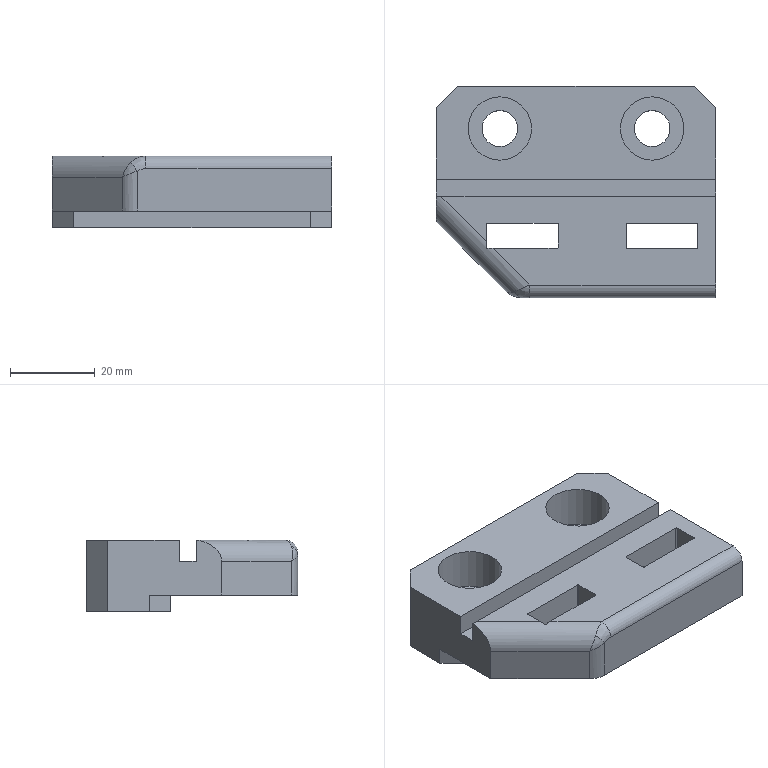Part | STEP file | gslz 2016.10.28-13_id326_x_t | 1 solid | 44 faces | box 66 x 50 x 17 mm | volume 37009 mm3 | plane 27 | cylinder 15 | spline 2 | commonest cylinder face diameters 0.6 x8 8.5 x2 10 x2 15 x2 6 x1